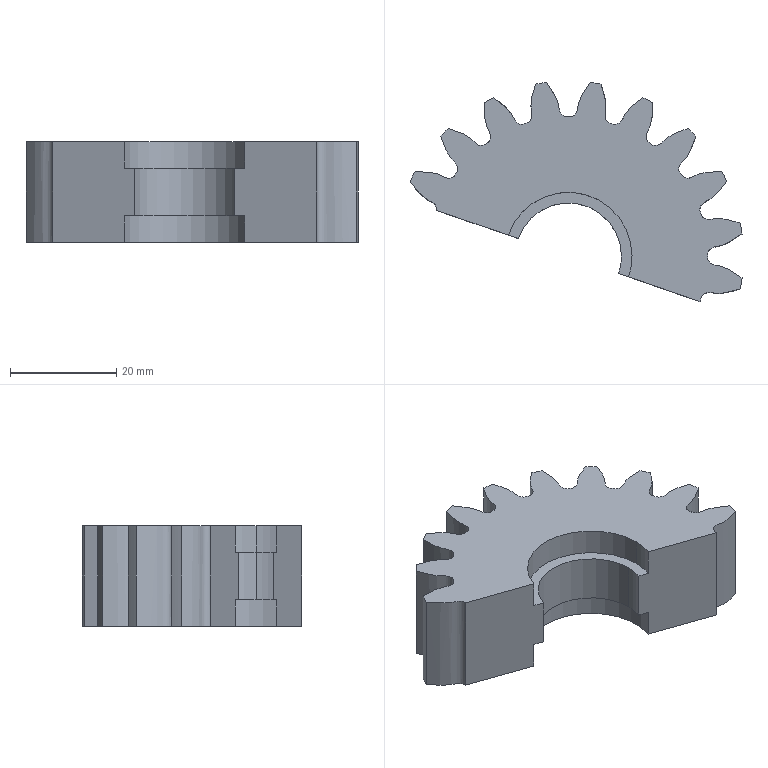Part | STEP file | Cuon T phu H01_18_Spur01 | 1 solid | 32 faces | box 62.602 x 41.333 x 19 mm | volume 22889 mm3 | cylinder 15 | spline 11 | plane 6 | commonest cylinder face diameters 66 x10 24 x3 20 x2